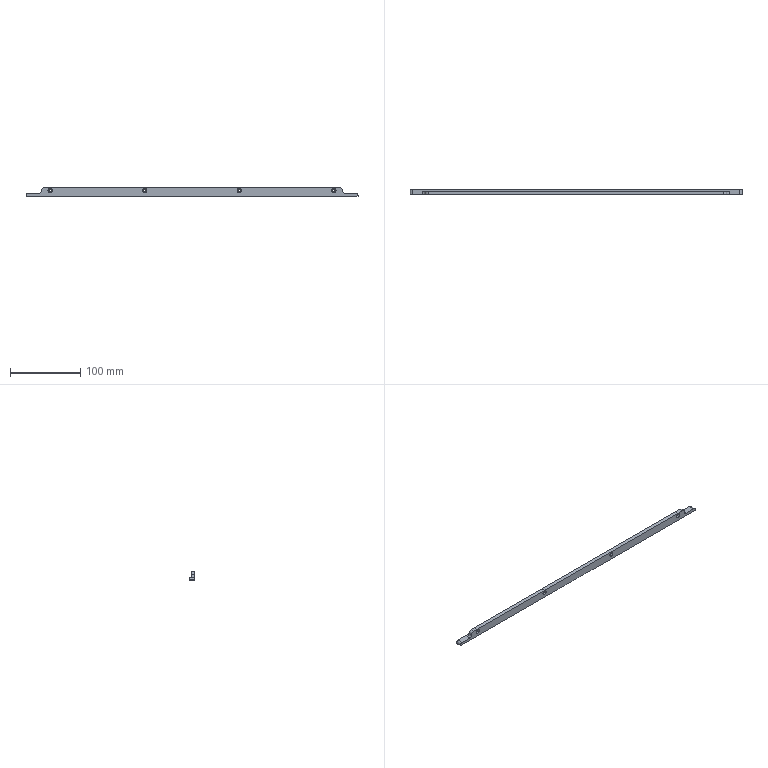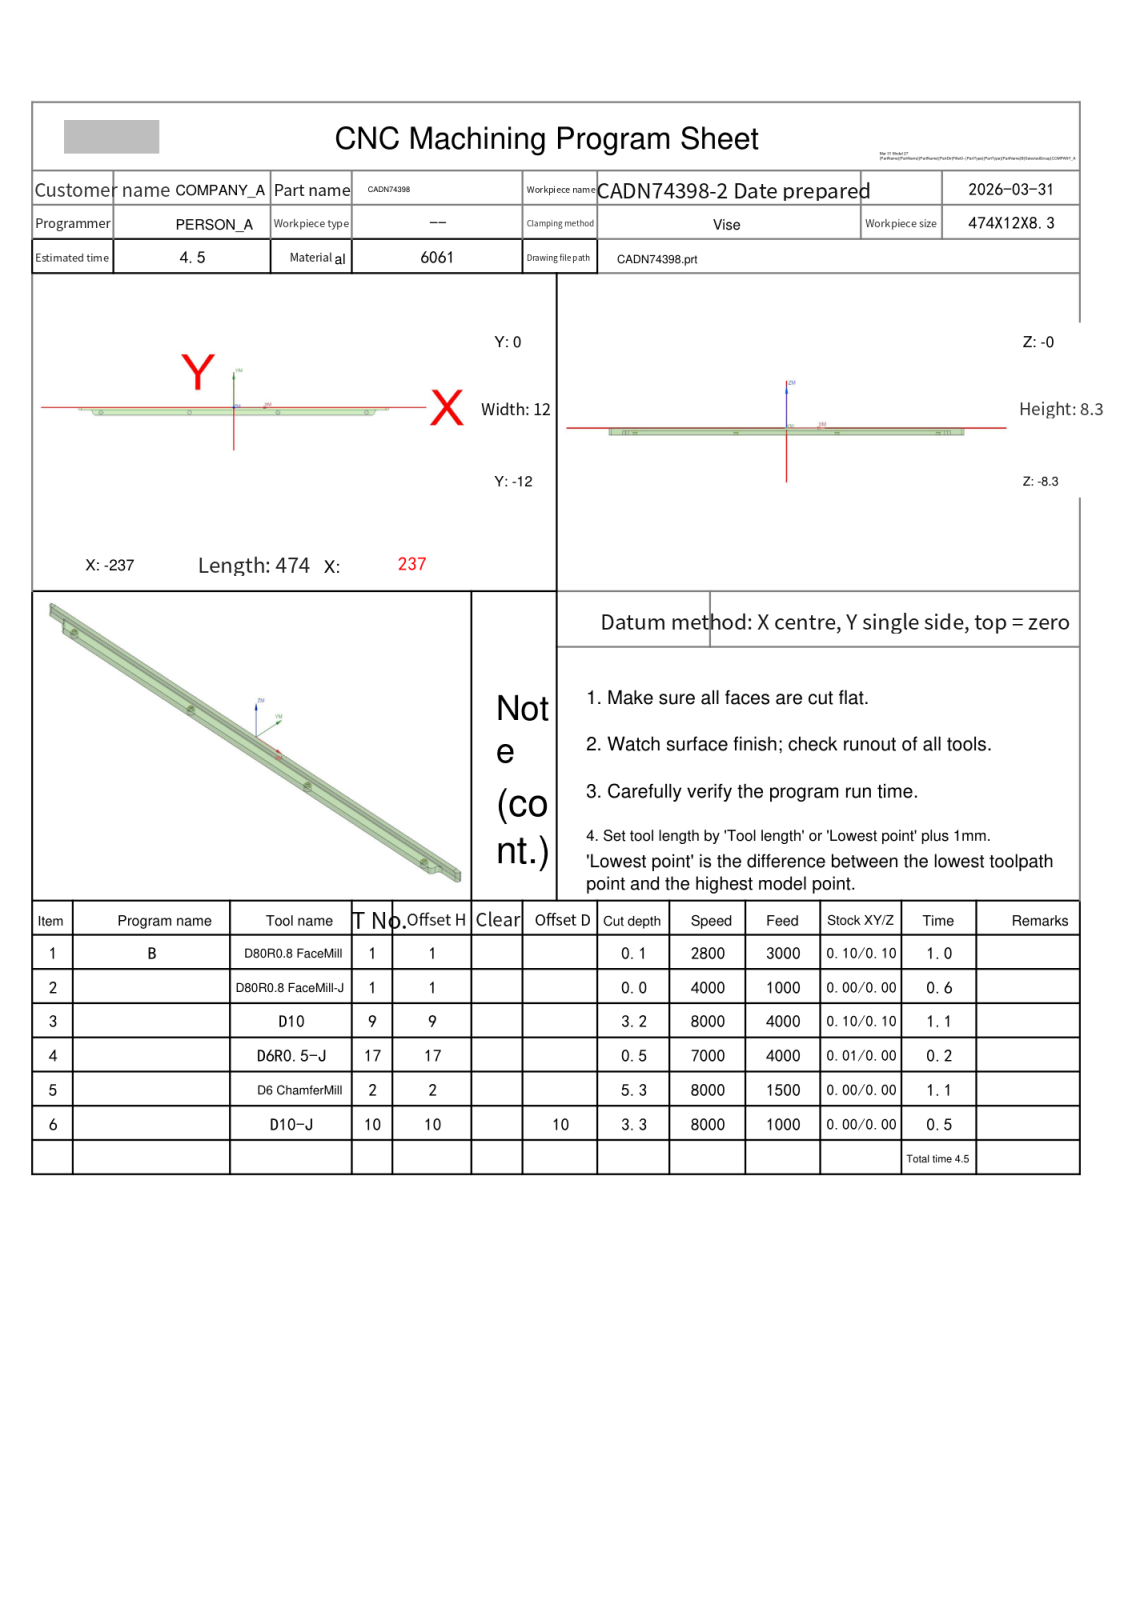NC program | NX | posted by the shop | part box 474 x 8.3 x 12 mm
Whole program:
%
O0001
(Machine time: 5.60 MIN)
(===Total Tool:5===)
(T1=D80R0.8 FaceMill D=80.  R=0.8  D-  H01 Z=0.    )
(T9=D10     D=10.  R=0.   D-  H09 Z=-3.2  )
(T17=D6R0.5-J D=6.   R=0.5  D-  H17 Z=-0.48 )
(T2=D6 ChamferMill   D=6.   R=0.   D-  H02 Z=-5.3  )
(T10=D10-J  D=10.  R=0.   D10 H10 Z=-3.3  )
G80 G90 G17 G49 G40
G91 G28 Z0
M01
N1 T01 M06
(D80R0.8 FaceMill  D=80. R=0.8 H=01 ce=0.10 di=0.10)
G00 G90 G54 X289.075 Y-2.571 M03 S2800
G43 H01 Z20.
M08
Z3.525
G01 Z1.525 F3000.
X277.063 Y-2.707
X-276.35 Y-8.989
X-288.494 Y-9.127
Z3.525
G00 X289.075 Y-2.571
Z3.05
G01 Z1.05
X277.063 Y-2.707
X-276.35 Y-8.989
X-288.494 Y-9.127
Z3.05
G00 X289.075 Y-2.571
Z2.575
G01 Z.575
X277.063 Y-2.707
X-276.35 Y-8.989
X-288.494 Y-9.127
Z2.575
G00 X289.075 Y-2.571
Z2.1
G01 Z.1
X277.063 Y-2.707
X-276.35 Y-8.989
X-288.494 Y-9.127
Z2.1
G00 Z20.
G91 G28 Z0.0
M05
M09
G91 G28 Z0.0
M01
N2 T01 M06
(D80R0.8 FaceMill-J  D=80. R=0.8 H=01 ce=0.00 di=0.00)
G00 G90 G54 X288.976 Y-2.581 M03 S4000
G43 H01 Z20.
M08
Z2.
G01 Z0.0 F1000.
X276.965 Y-2.717
X-276.252 Y-8.98
X-288.397 Y-9.118
Z2.
G00 Z20.
G91 G28 Z0.0
M05
M09
G91 G28 Z0.0
M01
N3 T09 M06
(D10  D=10. R=0. H=09 ce=0.10 di=0.10)
G00 G90 G54 X-219.369 Y-16.6 M03 S8000
G43 H09 Z11.5
M08
Z.62
G01 Z-.88 F4000.
X-213.291
X213.194
X213.295 Y-16.615
X213.392 Y-16.58
G03 X220.456 Y-10.882 I-1.982 J9.684
X220.832 Y-10.1 I-.624 J.782
X219.832 Y-9.1 I-1. J0.0
G01 X-219.832
X-222.832
Y-12.1
Z.62
G00 X-219.369 Y-16.6
Z.04
G01 Z-1.46
X-213.291
X213.194
X213.295 Y-16.615
X213.392 Y-16.58
G03 X220.456 Y-10.882 I-1.982 J9.684
X220.832 Y-10.1 I-.624 J.782
X219.832 Y-9.1 I-1. J0.0
G01 X-219.832
X-222.832
Y-12.1
Z.04
G00 X-219.369 Y-16.6
Z-.54
G01 Z-2.04
X-213.291
X213.194
X213.295 Y-16.615
X213.392 Y-16.58
G03 X220.456 Y-10.882 I-1.982 J9.684
X220.832 Y-10.1 I-.624 J.782
X219.832 Y-9.1 I-1. J0.0
G01 X-219.832
X-222.832
Y-12.1
Z-.54
G00 X-219.369 Y-16.6
Z-1.12
G01 Z-2.62
X-213.291
X213.194
X213.295 Y-16.615
X213.392 Y-16.58
G03 X220.456 Y-10.882 I-1.982 J9.684
X220.832 Y-10.1 I-.624 J.782
X219.832 Y-9.1 I-1. J0.0
G01 X-219.832
X-222.832
Y-12.1
Z-1.12
G00 X-219.369 Y-16.6
Z-1.7
G01 Z-3.2
X-213.291
X213.194
X213.295 Y-16.615
X213.392 Y-16.58
G03 X220.456 Y-10.882 I-1.982 J9.684
X220.832 Y-10.1 I-.624 J.782
X219.832 Y-9.1 I-1. J0.0
G01 X-219.832
X-222.832
Y-12.1
Z-1.7
G00 Z11.5
G91 G28 Z0.0
M05
M09
G91 G28 Z0.0
M01
N4 T17 M06
(D6R0.5-J  D=6. R=0.5 H=17 ce=0.01 di=0.00)
G00 G90 G54 X234.626 Y6.016 M03 S7000
G43 H17 Z11.5
M08
Z.492
G01 Z-.008 F4000.
X234.629 Y1.074
X234.63 Y0.0
Y-4.
X234.627 Y-5.07
X234.679 Z-.012
X234.726 Z-.016
X234.729 Y-4.
Y0.0
Y1.074
X234.779 Z-.02
X234.828 Y1.075 Z-.024
X234.829 Y0.0
Y-4.
X234.826 Y-5.07
X234.879 Z-.028
X234.926 Z-.032
X234.929 Y-4.
Y0.0
X234.928 Y1.075
X234.979 Z-.036
X235.028 Z-.04
Y0.0
Y-4.
X235.025 Y-5.069
X235.078 Z-.044
X235.125 Z-.048
X235.128 Y-4.
Y0.0
X235.127 Y1.076
X235.178 Z-.052
X235.227 Z-.056
X235.228 Y0.0
Y-4.
X235.225 Y-5.069
X235.278 Z-.06
X235.324 Z-.064
X235.327 Y-4.
Y0.0
Y1.076
X235.377 Z-.068
X235.427 Z-.072
Y0.0
Y-4.
X235.424 Y-5.069
X235.477 Z-.076
X235.524 Z-.08
X235.527 Y-4.
Y0.0
X235.526 Y1.077
X235.577 Z-.084
X235.626 Z-.088
Y0.0
Y-4.
X235.623 Y-5.068
X235.676 Z-.092
X235.723 Y-5.067 Z-.096
X235.726 Y-4.
Y0.0
Y1.077
X235.776 Y1.078 Z-.1
X235.825 Z-.104
X235.826 Y0.0
Y-4.
X235.823 Y-5.066
X235.876 Z-.108
X235.923 Y-5.065 Z-.112
X235.926 Y-4.
Y0.0
X235.925 Y1.078
X235.975 Z-.116
X236.025 Z-.12
Y0.0
Y-4.
X236.022 Y-5.064
X236.075 Z-.124
X236.122 Z-.128
X236.125 Y-4.
Y0.0
X236.124 Y1.079
X236.175 Z-.132
X236.224 Z-.136
X236.225 Y0.0
Y-4.
X236.222 Y-5.063
X236.274 Y-5.062 Z-.14
X236.323 Z-.144
X236.324 Y-4.
Y0.0
Y1.079
X236.374 Z-.148
X236.423 Z-.152
X236.424 Y0.0
Y-4.
X236.421 Y-5.06
X236.474 Y-5.059 Z-.156
X236.521 Y-5.058 Z-.159
X236.524 Y-4.
Y0.0
X236.523 Y1.079
X236.573 Z-.163
X236.623 Z-.167
Y0.0
Y-3.998
X236.62 Y-5.057
X236.673 Y-5.054 Z-.171
X236.72 Y-5.052 Z-.175
X236.723 Y-3.995
Y0.0
X236.722 Y1.079
X236.773 Z-.179
X236.822 Z-.183
X236.823 Y0.0
Y-3.988
X236.82 Y-5.045
X236.872 Y-5.041 Z-.187
X236.92 Y-5.037 Z-.191
X236.922 Y-3.976
Y0.0
Y1.079
X236.972 Z-.195
X237.021 Z-.199
X237.022 Y0.0
Y-3.963
X237.02 Y-5.03
X237.072 Y-5.022 Z-.203
X237.12 Y-5.015 Z-.207
X237.122 Y-3.945
Y0.0
X237.121 Y1.079
X237.172 Z-.211
X237.221 Z-.215
Y0.0
Y-3.924
Y-5.001
X237.271 Y-4.992 Z-.219
X237.321 Y-4.984 Z-.223
Y-3.9
Y0.0
Y1.079
X237.371 Z-.227
X237.42 Z-.231
X237.421 Y0.0
Y-3.871
X237.42 Y-4.961
X237.52 Y-4.936 Z-.239
Y-3.838
Y0.0
Y1.079
X237.57 Z-.243
X237.62 Z-.247
Y0.0
Y-3.802
X237.619 Y-4.911
X237.718 Y-4.885 Z-.255
X237.72 Y-3.762
Y0.0
X237.719 Y1.079
X237.77 Z-.259
X237.819 Z-.263
Y0.0
Y-3.718
X237.817 Y-4.851
X237.916 Y-4.816 Z-.271
X237.919 Y-3.669
Y0.0
Y1.079
X237.969 Z-.275
X238.018 Z-.279
X238.019 Y0.0
Y-3.615
X238.015 Y-4.782
X238.115 Y-4.741 Z-.287
X238.119 Y-3.557
Y0.0
X238.118 Y1.078
X238.168 Z-.291
X238.218 Z-.295
Y0.0
Y-3.493
X238.216 Y-4.697
X238.318 Y-4.652 Z-.303
Y-3.423
Y0.0
X238.317 Y1.078
X238.368 Y1.077 Z-.307
X238.417 Z-.311
X238.418 Y0.0
Y-3.346
X238.417 Y-4.603
X238.514 Y-4.545 Z-.319
X238.517 Y-3.264
Y0.0
Y1.077
X238.567 Z-.323
X238.616 Z-.327
X238.617 Y0.0
Y-3.173
X238.613 Y-4.487
X238.713 Y-4.428 Z-.335
X238.717 Y-3.074
Y0.0
X238.716 Y1.076
X238.766 Z-.339
X238.816 Z-.343
Y0.0
Y-2.965
X238.813 Y-4.364
X238.915 Y-4.296 Z-.351
X238.916 Y-2.844
Y0.0
X238.915 Y1.076
X238.966 Z-.355
X239.015 Z-.359
X239.016 Y0.0
Y-2.709
X239.014 Y-4.219
X239.112 Y-4.141 Z-.367
X239.115 Y-2.555
Y0.0
Y1.075
X239.165 Z-.371
X239.214 Z-.375
X239.215 Y0.0
Y-2.377
X239.21 Y-4.054
X239.315 Y-3.968 Z-.383
Y-2.164
Y0.0
X239.314 Y1.074
X239.365 Z-.387
X239.414 Z-.391
Y0.0
Y-1.889
X239.413 Y-3.873
X239.508 Y-3.768 Z-.399
X239.516 Y-1.587
X239.514 Y-1.461
Y0.0
X239.513 Y1.074
X239.564 Z-.403
X239.613 Z-.407
X239.611 Y-3.659
X239.711 Y-3.538 Z-.415
X239.713 Y1.073
X239.763 Z-.419
X239.812 Z-.423
X239.808 Y-3.408
X239.863 Y-3.336 Z-.427
X239.911 Y-3.264 Z-.431
X239.912 Y1.073
X239.963 Y1.072 Z-.435
X240.012 Z-.439
Y-2.95
X240.005 Y-3.101
X240.062 Y-3.02 Z-.443
X240.112 Y-2.938 Z-.447
X240.111 Y1.072
X240.162 Z-.451
X240.211 Z-.455
X240.212 Y-2.609
X240.205 Y-2.736
X240.262 Y-2.623 Z-.459
X240.301 Y-2.508 Z-.463
X240.312 Y-2.269
X240.311 Y1.071
X240.361 Z-.467
X240.41 Z-.47
Y-2.242
G00 Z.022
X240.498 Y-8.446
G01 Z-.478
X240.506 Y-1.865
X240.509 Y1.011
G00 Z11.5
X-234.612 Y-10.026
Z.492
G01 Z-.008
X-234.627 Y-5.07
X-234.63 Y-4.
Y0.0
X-234.629 Y1.074
X-234.679 Z-.012
X-234.729 Z-.016
Y0.0
Y-4.
X-234.726 Y-5.07
X-234.779 Z-.02
X-234.826 Z-.024
X-234.829 Y-4.
Y0.0
X-234.828 Y1.075
X-234.879 Z-.028
X-234.928 Z-.032
X-234.929 Y0.0
Y-4.
X-234.926 Y-5.07
X-234.979 Z-.036
X-235.025 Y-5.069 Z-.04
X-235.028 Y-4.
Y0.0
Y1.075
X-235.078 Z-.044
X-235.127 Y1.076 Z-.048
X-235.128 Y0.0
Y-4.
X-235.125 Y-5.069
X-235.178 Z-.052
X-235.225 Z-.056
X-235.228 Y-4.
Y0.0
X-235.227 Y1.076
X-235.278 Z-.06
X-235.327 Z-.064
Y0.0
Y-4.
X-235.324 Y-5.069
X-235.377 Z-.068
X-235.424 Z-.072
X-235.427 Y-4.
Y0.0
Y1.076
X-235.477 Y1.077 Z-.076
X-235.526 Z-.08
X-235.527 Y0.0
Y-4.
X-235.524 Y-5.069
X-235.577 Y-5.068 Z-.084
X-235.623 Z-.088
X-235.626 Y-4.
Y0.0
Y1.077
X-235.676 Z-.092
X-235.726 Z-.096
Y0.0
Y-4.
X-235.723 Y-5.067
X-235.776 Z-.1
X-235.823 Y-5.066 Z-.104
X-235.826 Y-4.
Y0.0
X-235.825 Y1.078
X-235.876 Z-.108
X-235.925 Z-.112
X-235.926 Y0.0
Y-4.
X-235.923 Y-5.065
X-235.975 Z-.116
X-236.022 Y-5.064 Z-.12
X-236.025 Y-4.
Y0.0
Y1.078
X-236.075 Y1.079 Z-.124
X-236.124 Z-.128
X-236.125 Y0.0
Y-4.
X-236.122 Y-5.064
X-236.175 Y-5.063 Z-.132
X-236.222 Z-.136
X-236.225 Y-4.
Y0.0
X-236.224 Y1.079
X-236.274 Z-.14
X-236.324 Z-.144
Y0.0
Y-4.
X-236.323 Y-5.062
X-236.374 Y-5.061 Z-.148
X-236.421 Y-5.06 Z-.152
X-236.424 Y-4.
Y0.0
X-236.423 Y1.079
X-236.474 Z-.156
X-236.523 Z-.159
X-236.524 Y0.0
Y-4.
X-236.521 Y-5.058
X-236.573 Z-.163
X-236.62 Y-5.057 Z-.167
X-236.623 Y-3.998
Y0.0
Y1.079
X-236.673 Z-.171
X-236.722 Z-.175
X-236.723 Y0.0
Y-3.995
X-236.72 Y-5.052
X-236.773 Y-5.048 Z-.179
X-236.82 Y-5.045 Z-.183
X-236.823 Y-3.988
Y0.0
X-236.822 Y1.079
X-236.872 Z-.187
X-236.922 Z-.191
Y0.0
Y-3.976
X-236.92 Y-5.037
X-236.972 Y-5.033 Z-.195
X-237.02 Y-5.03 Z-.199
X-237.022 Y-3.963
Y0.0
X-237.021 Y1.079
X-237.072 Z-.203
X-237.121 Z-.207
X-237.122 Y0.0
Y-3.945
X-237.12 Y-5.015
X-237.172 Y-5.008 Z-.211
X-237.221 Y-5.001 Z-.215
Y-3.924
Y0.0
Y1.079
X-237.271 Z-.219
X-237.321 Z-.223
Y0.0
Y-3.899
Y-4.984
X-237.371 Y-4.972 Z-.227
X-237.42 Y-4.961 Z-.231
X-237.421 Y-3.871
Y0.0
X-237.42 Y1.079
X-237.471 Z-.235
X-237.52 Z-.239
Y0.0
Y-3.838
Y-4.936
X-237.619 Y-4.911 Z-.247
X-237.62 Y-3.802
Y0.0
Y1.079
X-237.67 Z-.251
X-237.719 Z-.255
X-237.72 Y0.0
Y-3.762
X-237.718 Y-4.885
X-237.817 Y-4.851 Z-.263
X-237.819 Y-3.718
Y0.0
Y1.079
X-237.869 Z-.267
X-237.919 Z-.271
Y0.0
Y-3.669
X-237.916 Y-4.816
X-238.015 Y-4.782 Z-.279
X-238.019 Y-3.615
Y0.0
X-238.018 Y1.079
X-238.069 Y1.078 Z-.283
X-238.118 Z-.287
X-238.119 Y0.0
Y-3.557
X-238.115 Y-4.741
X-238.216 Y-4.697 Z-.295
X-238.218 Y-3.493
Y0.0
Y1.078
X-238.268 Z-.299
X-238.317 Z-.303
X-238.318 Y0.0
Y-3.423
Y-4.652
X-238.417 Y-4.603 Z-.311
X-238.418 Y-3.346
Y0.0
X-238.417 Y1.077
X-238.467 Z-.315
X-238.517 Z-.319
Y0.0
Y-3.264
X-238.514 Y-4.545
X-238.613 Y-4.487 Z-.327
X-238.617 Y-3.173
Y0.0
X-238.616 Y1.077
X-238.667 Z-.331
X-238.716 Y1.076 Z-.335
X-238.717 Y0.0
Y-3.074
X-238.713 Y-4.428
X-238.813 Y-4.364 Z-.343
X-238.816 Y-2.965
Y0.0
Y1.076
X-238.866 Z-.347
X-238.915 Z-.351
X-238.916 Y0.0
Y-2.844
X-238.915 Y-4.296
X-239.014 Y-4.22 Z-.359
X-239.016 Y-2.709
Y0.0
X-239.015 Y1.076
X-239.065 Y1.075 Z-.363
X-239.115 Z-.367
Y0.0
Y-2.555
X-239.112 Y-4.141
X-239.21 Y-4.054 Z-.375
X-239.215 Y-2.378
Y0.0
X-239.214 Y1.075
X-239.265 Z-.379
X-239.314 Y1.074 Z-.383
X-239.315 Y0.0
Y-2.164
Y-3.968
X-239.413 Y-3.873 Z-.391
X-239.414 Y-1.889
Y0.0
Y1.074
X-239.464 Z-.395
X-239.513 Z-.399
X-239.514 Y0.0
Y-1.461
X-239.516 Y-1.587
X-239.508 Y-3.768
X-239.611 Y-3.659 Z-.407
X-239.613 Y1.074
X-239.664 Y1.073 Z-.411
X-239.713 Z-.415
X-239.711 Y-3.538
X-239.808 Y-3.408 Z-.423
X-239.812 Y1.073
X-239.863 Z-.427
X-239.912 Z-.431
X-239.911 Y-3.264
X-239.963 Y-3.183 Z-.435
X-240.005 Y-3.101 Z-.439
X-240.012 Y-2.95
Y1.072
X-240.062 Z-.443
X-240.111 Z-.447
X-240.112 Y-2.938
X-240.162 Y-2.837 Z-.451
X-240.205 Y-2.736 Z-.455
X-240.212 Y-2.609
X-240.211 Y1.072
X-240.262 Y1.071 Z-.459
X-240.311 Z-.463
X-240.312 Y-2.269
X-240.301 Y-2.508
X-240.361 Y-2.375 Z-.467
X-240.41 Y-2.242 Z-.47
Y1.071
X-240.509 Y1.011 Z-.478
X-240.506 Y-1.864
G00 Z11.5
G91 G28 Z0.0
M05
M09
G91 G28 Z0.0
M01
N5 T02 M06
(D6 ChamferMill  D=6. R=0. H=02 ce=0.00 di=0.00)
G00 G90 G54 X-202.5 Y-8. M03 S8000
G43 H02 Z20.
M08
G98 G81 X-202.5 Y-8. Z-5.3 R-.3 F1000.
X-67.5
X67.5
X202.5
G80
G00 Z20.
G00 G90 X232.349 Y-4.928 M03 S6500
Z20.
Z2.8
G01 Z-1.2 F1500.
X232.259 Y-4.966
X232. Y-5.
X-232.
X-232.259 Y-4.966
X-232.349 Y-4.928
Z2.8
G00 Y.928
G01 Z-1.2
X-232.259 Y.966
X-232. Y1.
X0.0
X232.
X232.259 Y.966
X232.349 Y.928
Z2.8
G00 Z10.
X216.161 Y-7.209
Z-1.81
G01 Z-4.5
X216.109 Y-7.255
X216.099 Y-7.273
X216.037 Y-7.531
X216. Y-8.
G02 X211. Y-13. I-5. J0.0
G01 X-211.
G02 X-216. Y-8. I0.0 J5.
G01 X-216.037 Y-7.531
X-216.099 Y-7.273
X-216.109 Y-7.255
X-216.161 Y-7.209
Z-1.81
G00 Z10.
X-202.088 Y-7.474
Z-2.076
G01 Z-4.5
G03 X-202.397 Y-7.314 I-1.075 J-1.687
G01 X-202.446 Y-7.29
X-202.5 Y-7.3
G03 X-203.2 Y-8. I0.0 J-.7
X-202.5 Y-8.7 I.7 J0.0
X-201.8 Y-8. I0.0 J.7
X-202.319 Y-7.324 I-.7 J0.0
G01 X-202.5 Y-7.3
X-202.554 Y-7.29
X-202.603 Y-7.314
G03 X-202.912 Y-7.474 I.765 J-1.848
G01 Z-2.076
G00 Z10.
X-67.088
Z-2.076
G01 Z-4.5
G03 X-67.397 Y-7.314 I-1.075 J-1.687
G01 X-67.446 Y-7.29
X-67.5 Y-7.3
G03 X-68.2 Y-8. I0.0 J-.7
X-67.5 Y-8.7 I.7 J0.0
X-66.8 Y-8. I0.0 J.7
X-67.319 Y-7.324 I-.7 J0.0
G01 X-67.5 Y-7.3
X-67.554 Y-7.29
X-67.603 Y-7.314
G03 X-67.912 Y-7.474 I.765 J-1.848
G01 Z-2.076
G00 Z10.
X67.912
Z-2.076
G01 Z-4.5
G03 X67.603 Y-7.314 I-1.075 J-1.687
G01 X67.554 Y-7.29
X67.5 Y-7.3
G03 X66.8 Y-8. I0.0 J-.7
X67.5 Y-8.7 I.7 J0.0
X68.2 Y-8. I0.0 J.7
X67.681 Y-7.324 I-.7 J0.0
G01 X67.5 Y-7.3
X67.446 Y-7.29
X67.397 Y-7.314
G03 X67.088 Y-7.474 I.765 J-1.848
G01 Z-2.076
G00 Z10.
X202.912
Z-2.076
G01 Z-4.5
G03 X202.603 Y-7.314 I-1.075 J-1.687
G01 X202.554 Y-7.29
X202.5 Y-7.3
G03 X201.8 Y-8. I0.0 J-.7
X202.5 Y-8.7 I.7 J0.0
X203.2 Y-8. I0.0 J.7
X202.681 Y-7.324 I-.7 J0.0
G01 X202.5 Y-7.3
X202.446 Y-7.29
X202.397 Y-7.314
G03 X202.088 Y-7.474 I.765 J-1.848
G01 Z-2.076
G00 Z20.
G91 G28 Z0.0
M05
M09
G91 G28 Z0.0
M01
N6 T10 M06
(D10-J  D=10. R=0. H=10 ce=0.00 di=0.00)
G00 G90 G54 X221.944 Y-11.2 M03 S8000
G43 H10 Z11.5
M08
Z-2.3
G01 Z-3.3 F1000.
G41 D10
Y-11.
G03 X219.944 Y-9. I-2. J0.0
G01 X-219.944
G03 X-221.944 Y-11. I0.0 J-2.
G01 G40 Y-11.2
Z-2.3
G00 Z11.5
M05
M09
G91 G28 Z0.0
G91 G28 Y0.0
M30
%